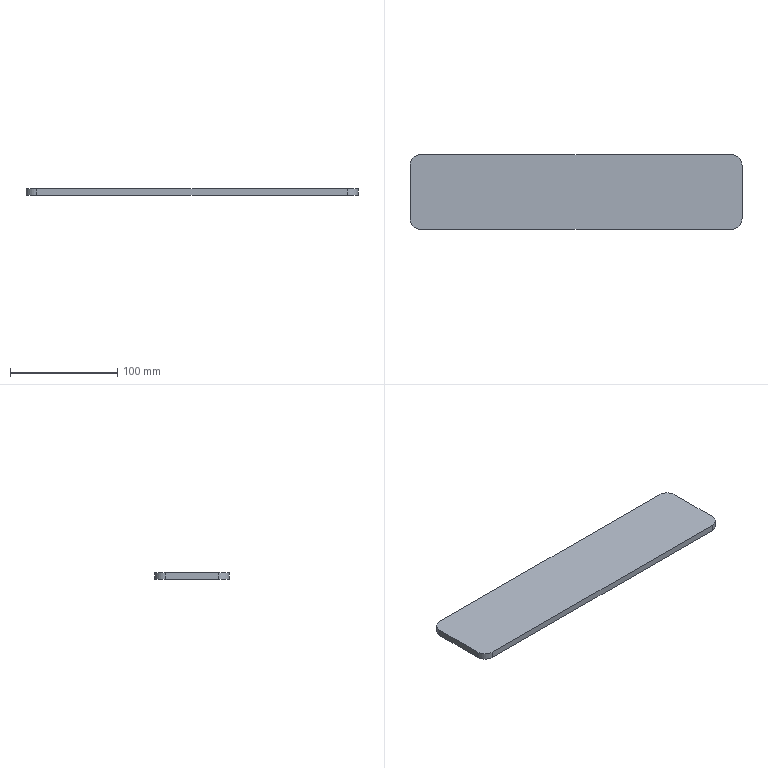Part | SolidWorks | features FlatPattern 1, SMBaseFlange 1, SheetMetal 1 | 1 solid | 10 faces | box 310 x 70 x 6 mm | volume 129685 mm3 | plane 6 | cylinder 4 | commonest cylinder face diameters 20 x4
STEP:
#1=CARTESIAN_POINT('',(100.,25.,0.));
#2=VERTEX_POINT('',#1);
#3=CARTESIAN_POINT('',(90.,35.,0.));
#4=VERTEX_POINT('',#3);
#5=CARTESIAN_POINT('',(90.,25.,0.));
#6=DIRECTION('',(0.,0.,1.));
#7=DIRECTION('',(1.,0.,0.));
#8=AXIS2_PLACEMENT_3D('',#5,#6,#7);
#9=CIRCLE('',#8,10.);
#10=EDGE_CURVE('',#2,#4,#9,.T.);
#11=ORIENTED_EDGE('',*,*,#10,.T.);
#12=CARTESIAN_POINT('',(90.,35.,6.));
#13=VERTEX_POINT('',#12);
#14=CARTESIAN_POINT('',(90.,35.,6.));
#15=DIRECTION('',(0.,0.,-1.));
#16=VECTOR('',#15,1000.);
#17=LINE('',#14,#16);
#18=EDGE_CURVE('',#13,#4,#17,.T.);
#19=ORIENTED_EDGE('',*,*,#18,.F.);
#20=CARTESIAN_POINT('',(100.,25.,6.));
#21=VERTEX_POINT('',#20);
#22=CARTESIAN_POINT('',(90.,25.,6.));
#23=DIRECTION('',(0.,0.,1.));
#24=DIRECTION('',(1.,0.,0.));
#25=AXIS2_PLACEMENT_3D('',#22,#23,#24);
#26=CIRCLE('',#25,10.);
#27=EDGE_CURVE('',#21,#13,#26,.T.);
#28=ORIENTED_EDGE('',*,*,#27,.F.);
#29=CARTESIAN_POINT('',(100.,25.,6.));
#30=DIRECTION('',(0.,0.,-1.));
#31=VECTOR('',#30,1000.);
#32=LINE('',#29,#31);
#33=EDGE_CURVE('',#21,#2,#32,.T.);
#34=ORIENTED_EDGE('',*,*,#33,.T.);
#35=EDGE_LOOP('',(#11,#19,#28,#34));
#36=FACE_OUTER_BOUND('',#35,.T.);
#37=CARTESIAN_POINT('',(90.,25.,6.));
#38=DIRECTION('',(0.,0.,-1.));
#39=DIRECTION('',(-1.,0.,0.));
#40=AXIS2_PLACEMENT_3D('',#37,#38,#39);
#41=CYLINDRICAL_SURFACE('',#40,10.);
#42=ADVANCED_FACE('',(#36),#41,.T.);
#43=CARTESIAN_POINT('',(-200.,35.,0.));
#44=VERTEX_POINT('',#43);
#45=CARTESIAN_POINT('',(90.,35.,0.));
#46=DIRECTION('',(-1.,0.,0.));
#47=VECTOR('',#46,1000.);
#48=LINE('',#45,#47);
#49=EDGE_CURVE('',#4,#44,#48,.T.);
#50=ORIENTED_EDGE('',*,*,#49,.T.);
#51=CARTESIAN_POINT('',(-200.,35.,6.));
#52=VERTEX_POINT('',#51);
#53=CARTESIAN_POINT('',(-200.,35.,6.));
#54=DIRECTION('',(0.,0.,-1.));
#55=VECTOR('',#54,1000.);
#56=LINE('',#53,#55);
#57=EDGE_CURVE('',#52,#44,#56,.T.);
#58=ORIENTED_EDGE('',*,*,#57,.F.);
#59=CARTESIAN_POINT('',(90.,35.,6.));
#60=DIRECTION('',(-1.,0.,0.));
#61=VECTOR('',#60,1000.);
#62=LINE('',#59,#61);
#63=EDGE_CURVE('',#13,#52,#62,.T.);
#64=ORIENTED_EDGE('',*,*,#63,.F.);
#65=ORIENTED_EDGE('',*,*,#18,.T.);
#66=EDGE_LOOP('',(#50,#58,#64,#65));
#67=FACE_OUTER_BOUND('',#66,.T.);
#68=CARTESIAN_POINT('',(90.,35.,6.));
#69=DIRECTION('',(0.,-1.,0.));
#70=DIRECTION('',(0.,0.,-1.));
#71=AXIS2_PLACEMENT_3D('',#68,#69,#70);
#72=PLANE('',#71);
#73=ADVANCED_FACE('',(#67),#72,.F.);
#74=CARTESIAN_POINT('',(-210.,25.,0.));
#75=VERTEX_POINT('',#74);
#76=CARTESIAN_POINT('',(-200.,25.,0.));
#77=DIRECTION('',(0.,0.,1.));
#78=DIRECTION('',(1.,0.,0.));
#79=AXIS2_PLACEMENT_3D('',#76,#77,#78);
#80=CIRCLE('',#79,10.);
#81=EDGE_CURVE('',#44,#75,#80,.T.);
#82=ORIENTED_EDGE('',*,*,#81,.T.);
#83=CARTESIAN_POINT('',(-210.,25.,6.));
#84=VERTEX_POINT('',#83);
#85=CARTESIAN_POINT('',(-210.,25.,6.));
#86=DIRECTION('',(0.,0.,-1.));
#87=VECTOR('',#86,1000.);
#88=LINE('',#85,#87);
#89=EDGE_CURVE('',#84,#75,#88,.T.);
#90=ORIENTED_EDGE('',*,*,#89,.F.);
#91=CARTESIAN_POINT('',(-200.,25.,6.));
#92=DIRECTION('',(0.,0.,1.));
#93=DIRECTION('',(1.,0.,0.));
#94=AXIS2_PLACEMENT_3D('',#91,#92,#93);
#95=CIRCLE('',#94,10.);
#96=EDGE_CURVE('',#52,#84,#95,.T.);
#97=ORIENTED_EDGE('',*,*,#96,.F.);
#98=ORIENTED_EDGE('',*,*,#57,.T.);
#99=EDGE_LOOP('',(#82,#90,#97,#98));
#100=FACE_OUTER_BOUND('',#99,.T.);
#101=CARTESIAN_POINT('',(-200.,25.,6.));
#102=DIRECTION('',(0.,0.,-1.));
#103=DIRECTION('',(-1.,0.,0.));
#104=AXIS2_PLACEMENT_3D('',#101,#102,#103);
#105=CYLINDRICAL_SURFACE('',#104,10.);
#106=ADVANCED_FACE('',(#100),#105,.T.);
#107=CARTESIAN_POINT('',(-210.,-25.,0.));
#108=VERTEX_POINT('',#107);
#109=CARTESIAN_POINT('',(-210.,25.,0.));
#110=DIRECTION('',(0.,-1.,0.));
#111=VECTOR('',#110,1000.);
#112=LINE('',#109,#111);
#113=EDGE_CURVE('',#75,#108,#112,.T.);
#114=ORIENTED_EDGE('',*,*,#113,.T.);
#115=CARTESIAN_POINT('',(-210.,-25.,6.));
#116=VERTEX_POINT('',#115);
#117=CARTESIAN_POINT('',(-210.,-25.,6.));
#118=DIRECTION('',(0.,0.,-1.));
#119=VECTOR('',#118,1000.);
#120=LINE('',#117,#119);
#121=EDGE_CURVE('',#116,#108,#120,.T.);
#122=ORIENTED_EDGE('',*,*,#121,.F.);
#123=CARTESIAN_POINT('',(-210.,25.,6.));
#124=DIRECTION('',(0.,-1.,0.));
#125=VECTOR('',#124,1000.);
#126=LINE('',#123,#125);
#127=EDGE_CURVE('',#84,#116,#126,.T.);
#128=ORIENTED_EDGE('',*,*,#127,.F.);
#129=ORIENTED_EDGE('',*,*,#89,.T.);
#130=EDGE_LOOP('',(#114,#122,#128,#129));
#131=FACE_OUTER_BOUND('',#130,.T.);
#132=CARTESIAN_POINT('',(-210.,25.,6.));
#133=DIRECTION('',(1.,0.,0.));
#134=DIRECTION('',(0.,0.,-1.));
#135=AXIS2_PLACEMENT_3D('',#132,#133,#134);
#136=PLANE('',#135);
#137=ADVANCED_FACE('',(#131),#136,.F.);
#138=CARTESIAN_POINT('',(-200.,-35.,0.));
#139=VERTEX_POINT('',#138);
#140=CARTESIAN_POINT('',(-200.,-25.,0.));
#141=DIRECTION('',(0.,0.,1.));
#142=DIRECTION('',(1.,0.,0.));
#143=AXIS2_PLACEMENT_3D('',#140,#141,#142);
#144=CIRCLE('',#143,10.);
#145=EDGE_CURVE('',#108,#139,#144,.T.);
#146=ORIENTED_EDGE('',*,*,#145,.T.);
#147=CARTESIAN_POINT('',(-200.,-35.,6.));
#148=VERTEX_POINT('',#147);
#149=CARTESIAN_POINT('',(-200.,-35.,6.));
#150=DIRECTION('',(0.,0.,-1.));
#151=VECTOR('',#150,1000.);
#152=LINE('',#149,#151);
#153=EDGE_CURVE('',#148,#139,#152,.T.);
#154=ORIENTED_EDGE('',*,*,#153,.F.);
#155=CARTESIAN_POINT('',(-200.,-25.,6.));
#156=DIRECTION('',(0.,0.,1.));
#157=DIRECTION('',(1.,0.,0.));
#158=AXIS2_PLACEMENT_3D('',#155,#156,#157);
#159=CIRCLE('',#158,10.);
#160=EDGE_CURVE('',#116,#148,#159,.T.);
#161=ORIENTED_EDGE('',*,*,#160,.F.);
#162=ORIENTED_EDGE('',*,*,#121,.T.);
#163=EDGE_LOOP('',(#146,#154,#161,#162));
#164=FACE_OUTER_BOUND('',#163,.T.);
#165=CARTESIAN_POINT('',(-200.,-25.,6.));
#166=DIRECTION('',(0.,0.,-1.));
#167=DIRECTION('',(-1.,0.,0.));
#168=AXIS2_PLACEMENT_3D('',#165,#166,#167);
#169=CYLINDRICAL_SURFACE('',#168,10.);
#170=ADVANCED_FACE('',(#164),#169,.T.);
#171=CARTESIAN_POINT('',(90.,-35.,0.));
#172=VERTEX_POINT('',#171);
#173=CARTESIAN_POINT('',(-200.,-35.,0.));
#174=DIRECTION('',(1.,0.,0.));
#175=VECTOR('',#174,1000.);
#176=LINE('',#173,#175);
#177=EDGE_CURVE('',#139,#172,#176,.T.);
#178=ORIENTED_EDGE('',*,*,#177,.T.);
#179=CARTESIAN_POINT('',(90.,-35.,6.));
#180=VERTEX_POINT('',#179);
#181=CARTESIAN_POINT('',(90.,-35.,6.));
#182=DIRECTION('',(0.,0.,-1.));
#183=VECTOR('',#182,1000.);
#184=LINE('',#181,#183);
#185=EDGE_CURVE('',#180,#172,#184,.T.);
#186=ORIENTED_EDGE('',*,*,#185,.F.);
#187=CARTESIAN_POINT('',(-200.,-35.,6.));
#188=DIRECTION('',(1.,0.,0.));
#189=VECTOR('',#188,1000.);
#190=LINE('',#187,#189);
#191=EDGE_CURVE('',#148,#180,#190,.T.);
#192=ORIENTED_EDGE('',*,*,#191,.F.);
#193=ORIENTED_EDGE('',*,*,#153,.T.);
#194=EDGE_LOOP('',(#178,#186,#192,#193));
#195=FACE_OUTER_BOUND('',#194,.T.);
#196=CARTESIAN_POINT('',(-200.,-35.,6.));
#197=DIRECTION('',(0.,1.,0.));
#198=DIRECTION('',(0.,0.,1.));
#199=AXIS2_PLACEMENT_3D('',#196,#197,#198);
#200=PLANE('',#199);
#201=ADVANCED_FACE('',(#195),#200,.F.);
#202=CARTESIAN_POINT('',(100.,-25.,0.));
#203=VERTEX_POINT('',#202);
#204=CARTESIAN_POINT('',(90.,-25.,0.));
#205=DIRECTION('',(0.,0.,1.));
#206=DIRECTION('',(-1.,0.,0.));
#207=AXIS2_PLACEMENT_3D('',#204,#205,#206);
#208=CIRCLE('',#207,10.);
#209=EDGE_CURVE('',#172,#203,#208,.T.);
#210=ORIENTED_EDGE('',*,*,#209,.T.);
#211=CARTESIAN_POINT('',(100.,-25.,6.));
#212=VERTEX_POINT('',#211);
#213=CARTESIAN_POINT('',(100.,-25.,6.));
#214=DIRECTION('',(0.,0.,-1.));
#215=VECTOR('',#214,1000.);
#216=LINE('',#213,#215);
#217=EDGE_CURVE('',#212,#203,#216,.T.);
#218=ORIENTED_EDGE('',*,*,#217,.F.);
#219=CARTESIAN_POINT('',(90.,-25.,6.));
#220=DIRECTION('',(0.,0.,1.));
#221=DIRECTION('',(-1.,0.,0.));
#222=AXIS2_PLACEMENT_3D('',#219,#220,#221);
#223=CIRCLE('',#222,10.);
#224=EDGE_CURVE('',#180,#212,#223,.T.);
#225=ORIENTED_EDGE('',*,*,#224,.F.);
#226=ORIENTED_EDGE('',*,*,#185,.T.);
#227=EDGE_LOOP('',(#210,#218,#225,#226));
#228=FACE_OUTER_BOUND('',#227,.T.);
#229=CARTESIAN_POINT('',(90.,-25.,6.));
#230=DIRECTION('',(0.,0.,-1.));
#231=DIRECTION('',(-1.,0.,0.));
#232=AXIS2_PLACEMENT_3D('',#229,#230,#231);
#233=CYLINDRICAL_SURFACE('',#232,10.);
#234=ADVANCED_FACE('',(#228),#233,.T.);
#235=CARTESIAN_POINT('',(100.,-25.,0.));
#236=DIRECTION('',(0.,1.,0.));
#237=VECTOR('',#236,1000.);
#238=LINE('',#235,#237);
#239=EDGE_CURVE('',#203,#2,#238,.T.);
#240=ORIENTED_EDGE('',*,*,#239,.T.);
#241=ORIENTED_EDGE('',*,*,#33,.F.);
#242=CARTESIAN_POINT('',(100.,-25.,6.));
#243=DIRECTION('',(0.,1.,0.));
#244=VECTOR('',#243,1000.);
#245=LINE('',#242,#244);
#246=EDGE_CURVE('',#212,#21,#245,.T.);
#247=ORIENTED_EDGE('',*,*,#246,.F.);
#248=ORIENTED_EDGE('',*,*,#217,.T.);
#249=EDGE_LOOP('',(#240,#241,#247,#248));
#250=FACE_OUTER_BOUND('',#249,.T.);
#251=CARTESIAN_POINT('',(100.,-25.,6.));
#252=DIRECTION('',(-1.,0.,0.));
#253=DIRECTION('',(0.,0.,1.));
#254=AXIS2_PLACEMENT_3D('',#251,#252,#253);
#255=PLANE('',#254);
#256=ADVANCED_FACE('',(#250),#255,.F.);
#257=ORIENTED_EDGE('',*,*,#27,.T.);
#258=ORIENTED_EDGE('',*,*,#63,.T.);
#259=ORIENTED_EDGE('',*,*,#96,.T.);
#260=ORIENTED_EDGE('',*,*,#127,.T.);
#261=ORIENTED_EDGE('',*,*,#160,.T.);
#262=ORIENTED_EDGE('',*,*,#191,.T.);
#263=ORIENTED_EDGE('',*,*,#224,.T.);
#264=ORIENTED_EDGE('',*,*,#246,.T.);
#265=EDGE_LOOP('',(#257,#258,#259,#260,#261,#262,#263,#264));
#266=FACE_OUTER_BOUND('',#265,.T.);
#267=CARTESIAN_POINT('',(90.,25.,6.));
#268=DIRECTION('',(0.,0.,1.));
#269=DIRECTION('',(1.,0.,0.));
#270=AXIS2_PLACEMENT_3D('',#267,#268,#269);
#271=PLANE('',#270);
#272=ADVANCED_FACE('',(#266),#271,.T.);
#273=ORIENTED_EDGE('',*,*,#10,.F.);
#274=ORIENTED_EDGE('',*,*,#239,.F.);
#275=ORIENTED_EDGE('',*,*,#209,.F.);
#276=ORIENTED_EDGE('',*,*,#177,.F.);
#277=ORIENTED_EDGE('',*,*,#145,.F.);
#278=ORIENTED_EDGE('',*,*,#113,.F.);
#279=ORIENTED_EDGE('',*,*,#81,.F.);
#280=ORIENTED_EDGE('',*,*,#49,.F.);
#281=EDGE_LOOP('',(#273,#274,#275,#276,#277,#278,#279,#280));
#282=FACE_OUTER_BOUND('',#281,.T.);
#283=CARTESIAN_POINT('',(90.,25.,0.));
#284=DIRECTION('',(0.,0.,1.));
#285=DIRECTION('',(1.,0.,0.));
#286=AXIS2_PLACEMENT_3D('',#283,#284,#285);
#287=PLANE('',#286);
#288=ADVANCED_FACE('',(#282),#287,.F.);
#289=CLOSED_SHELL('',(#42,#73,#106,#137,#170,#201,#234,#256,#272,#288));
#290=MANIFOLD_SOLID_BREP('',#289);
#291=CARTESIAN_POINT('',(0.,0.,0.));
#292=DIRECTION('',(0.,0.,1.));
#293=DIRECTION('',(1.,0.,0.));
#294=AXIS2_PLACEMENT_3D('',#291,#292,#293);
#295=(LENGTH_UNIT()NAMED_UNIT(*)SI_UNIT(.MILLI.,.METRE.));
#296=UNCERTAINTY_MEASURE_WITH_UNIT(LENGTH_MEASURE(0.00001),#295,'','');
#297=(NAMED_UNIT(*)PLANE_ANGLE_UNIT()SI_UNIT($,.RADIAN.));
#298=(NAMED_UNIT(*)SI_UNIT($,.STERADIAN.)SOLID_ANGLE_UNIT());
#299=(GEOMETRIC_REPRESENTATION_CONTEXT(3)GLOBAL_UNCERTAINTY_ASSIGNED_CONTEXT((#296))GLOBAL_UNIT_ASSIGNED_CONTEXT((#295,#297,#298))REPRESENTATION_CONTEXT('',''));
#300=ADVANCED_BREP_SHAPE_REPRESENTATION('',(#290,#294),#299);